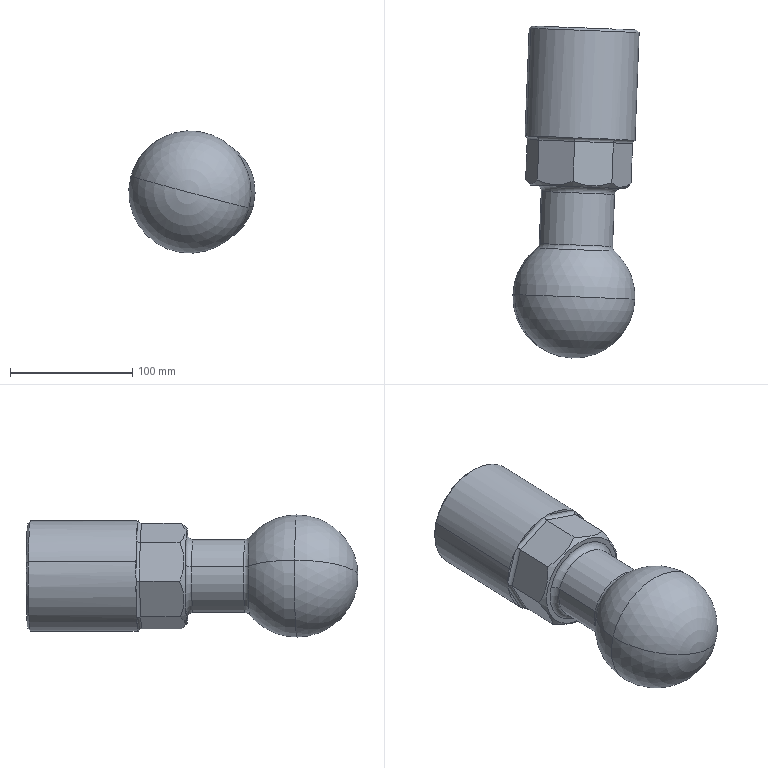Part | SolidWorks | features BaseBody 1 | 1 solid | 42 faces | box 103.341 x 271.49 x 100 mm | volume 1435475 mm3 | plane 17 | cylinder 12 | torus 4 | sphere 4 | spline 3 | cone 2 | commonest cylinder face diameters 6 x8 60 x2 90 x2